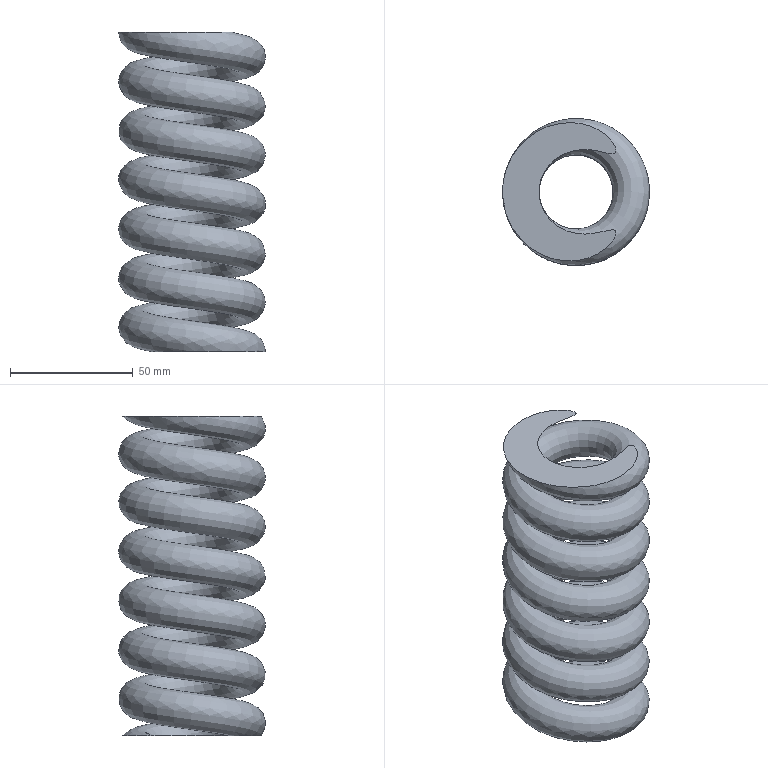Part | NX | features solid 2 | 1 solid | 3 faces | box 59.85 x 59.846 x 130 mm | volume 160730 mm3 | plane 2 | spline 1